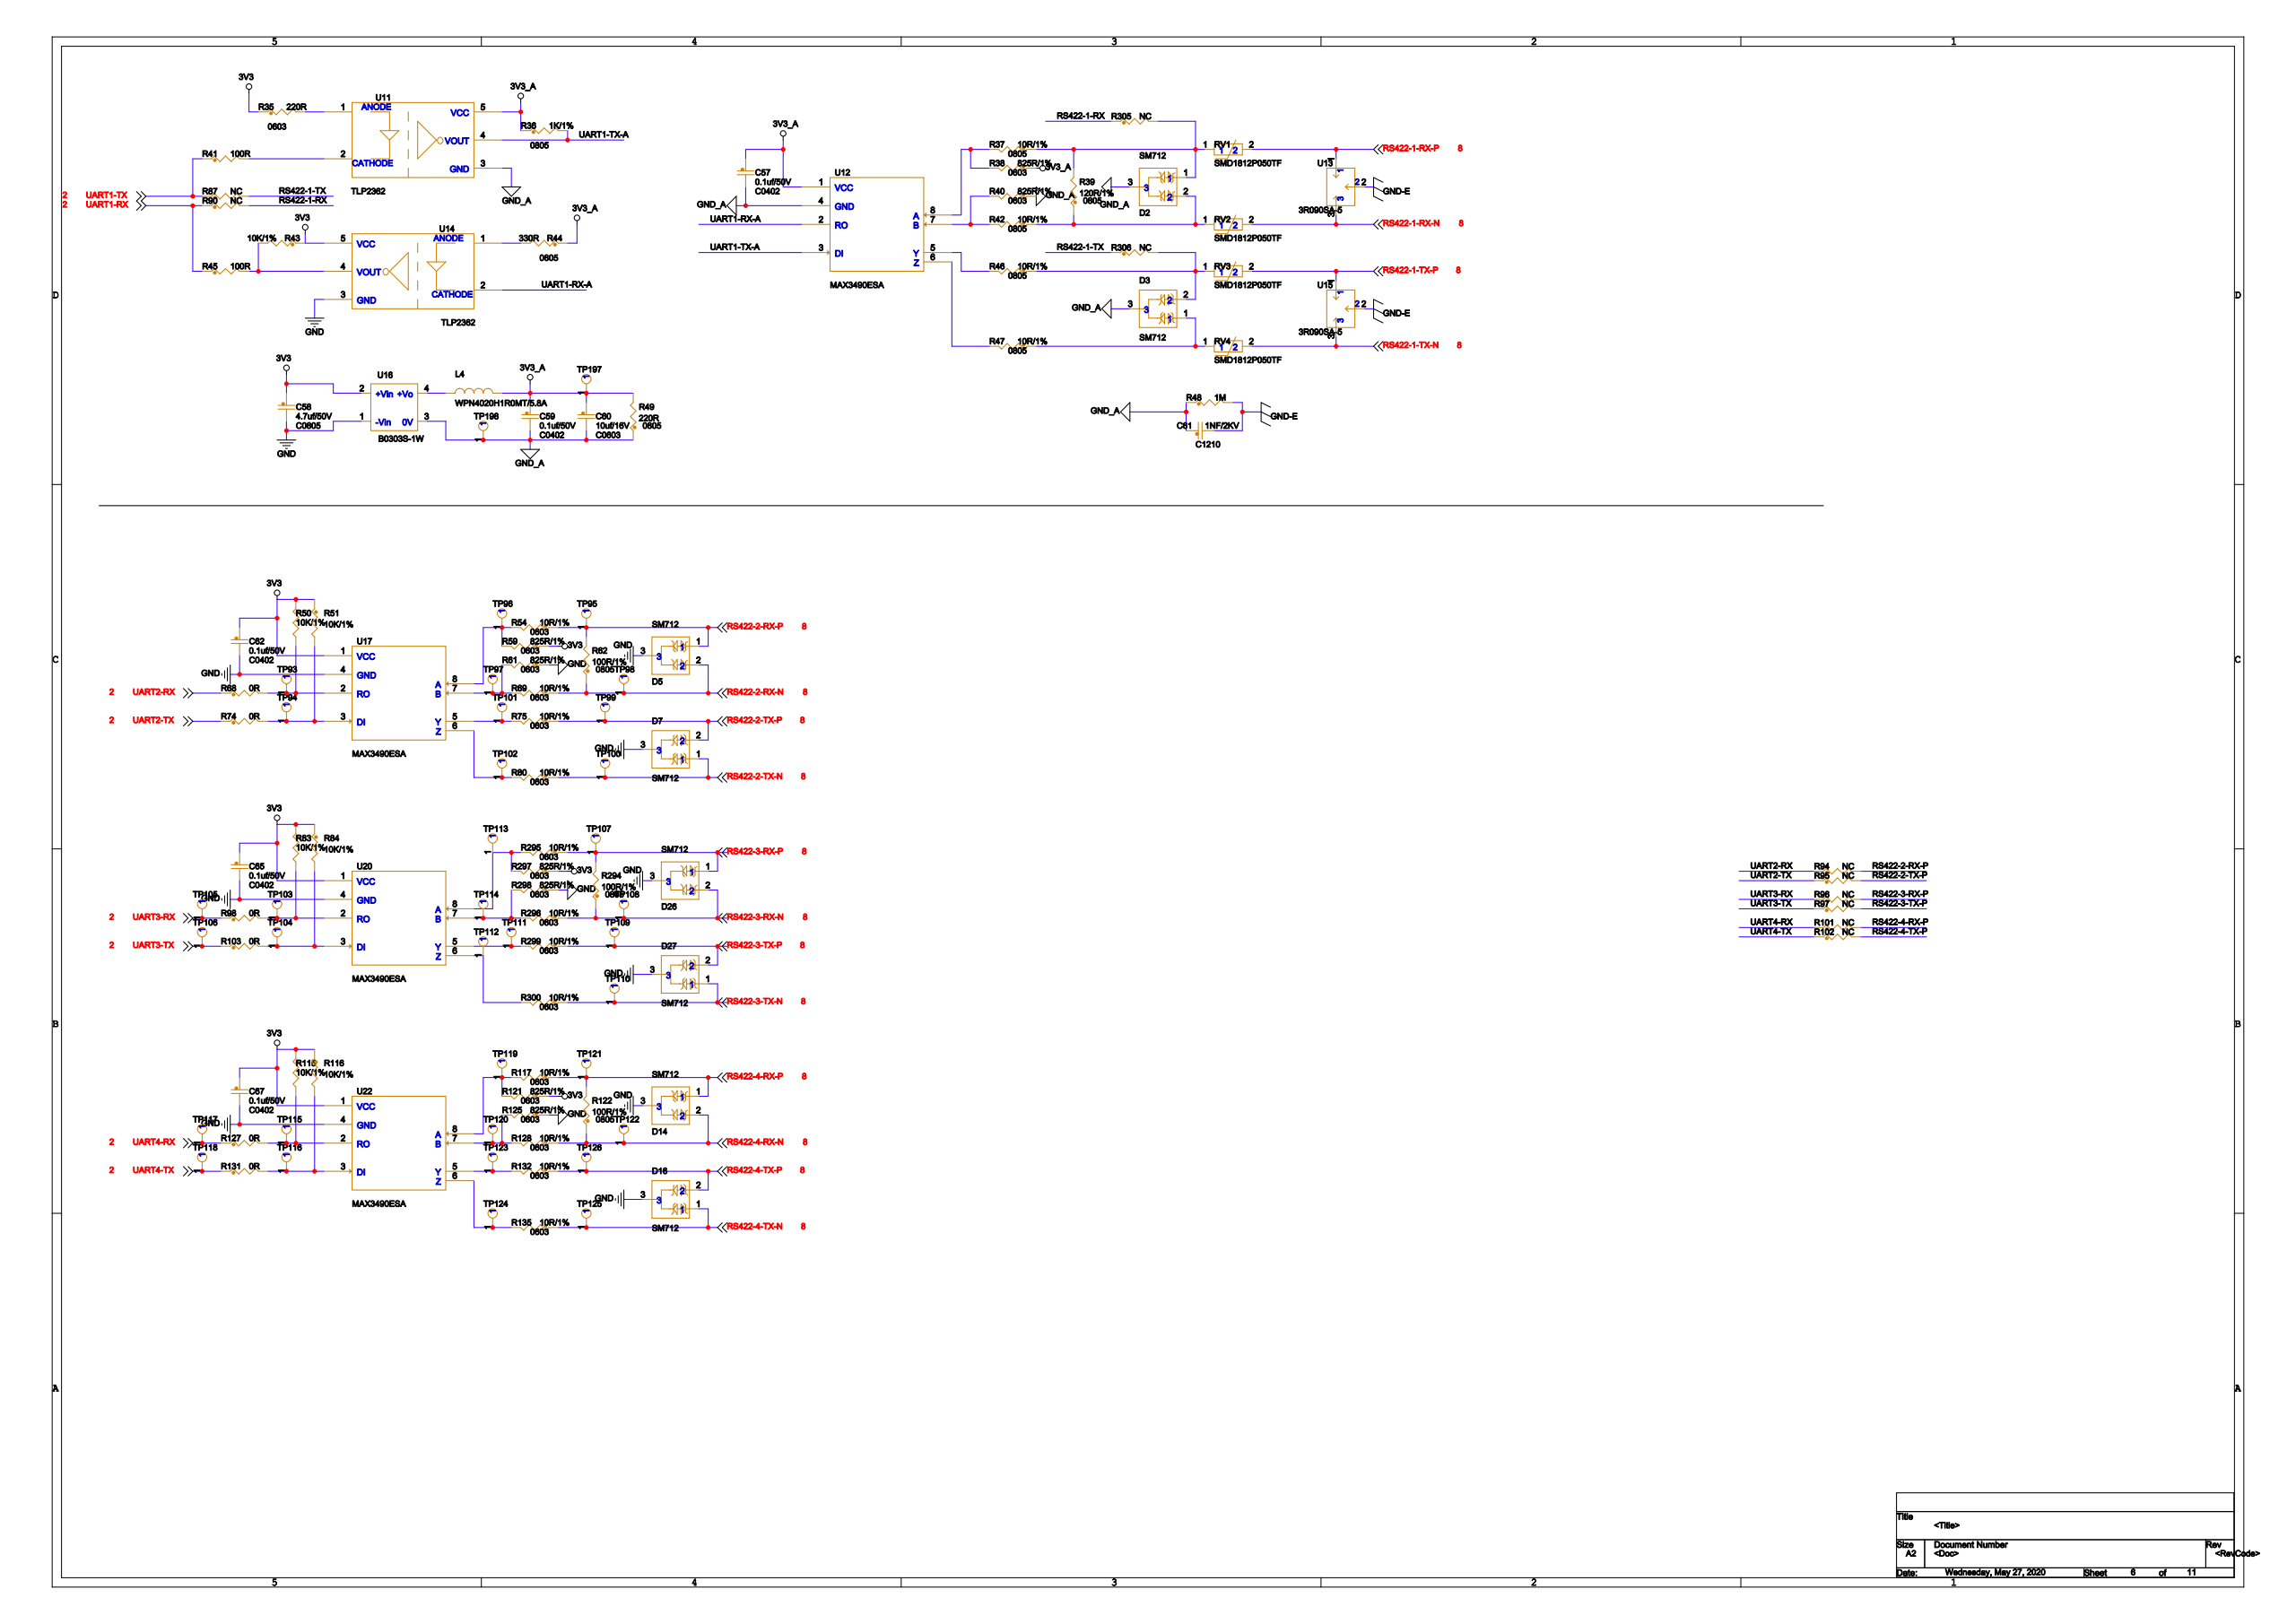Circuit board | Cadence Allegro | 521 parts | 239 nets | one sheet of the schematic
Parts on this sheet (reference | value | footprint):
C57 | 0.1uf/50V | C0402
C58 | 4.7uf/50V | C0805
C59 | 0.1uf/50V | C0402
C60 | 10uf/16V | C0603
C61 | 1NF/2KV | C1210
C62 | 0.1uf/50V | C0402
C65 | 0.1uf/50V | C0402
C67 | 0.1uf/50V | C0402
D2 | SM712 | SOT23
D3 | SM712 | SOT23
D5 | SM712 | SOT23
D7 | SM712 | SOT23
D14 | SM712 | SOT23
D16 | SM712 | SOT23
D26 | SM712 | SOT23
D27 | SM712 | SOT23
L4 | WPN4020H1R0MT/5.8A | SM_IND_4
R35 | 220R | 0603
R36 | 1K/1% | 0805
R37 | 10R/1% | 0805
R38 | 825R/1% | 0603
R39 | 120R/1% | 0805
R40 | 825R/1% | 0603
R41 | 100R | 0603
R42 | 10R/1% | 0805
R43 | 10K/1% | 0402
R44 | 330R | 0805
R45 | 100R | 0603
R46 | 10R/1% | 0805
R47 | 10R/1% | 0805
R48 | 1M | 1206
R49 | 220R | 0805
R50 | 10K/1% | 0402
R51 | 10K/1% | 0402
R54 | 10R/1% | 0603
R59 | 825R/1% | 0603
R61 | 825R/1% | 0603
R62 | 100R/1% | 0805
R68 | 0R | 0603
R69 | 10R/1% | 0603
R74 | 0R | 0603
R75 | 10R/1% | 0603
R80 | 10R/1% | 0603
R83 | 10K/1% | 0402
R84 | 10K/1% | 0402
R87 | NC | 0603
R90 | NC | 0603
R94 | NC | 0603
R95 | NC | 0603
R96 | NC | 0603
R97 | NC | 0603
R98 | 0R | 0603
R101 | NC | 0603
R102 | NC | 0603
R103 | 0R | 0603
R115 | 10K/1% | 0402
R116 | 10K/1% | 0402
R117 | 10R/1% | 0603
R121 | 825R/1% | 0603
R122 | 100R/1% | 0805
R125 | 825R/1% | 0603
R127 | 0R | 0603
R128 | 10R/1% | 0603
R131 | 0R | 0603
R132 | 10R/1% | 0603
R135 | 10R/1% | 0603
R294 | 100R/1% | 0805
R295 | 10R/1% | 0603
R296 | 10R/1% | 0603
R297 | 825R/1% | 0603
R298 | 825R/1% | 0603
R299 | 10R/1% | 0603
R300 | 10R/1% | 0603
R305 | NC | 0603
R306 | NC | 0603
RV1 | SMD1812P050TF | 1812_2
RV2 | SMD1812P050TF | 1812_2
RV3 | SMD1812P050TF | 1812_2
RV4 | SMD1812P050TF | 1812_2
TP93 | TESTPOINT | TESTPOINT-33MIL
TP94 | TESTPOINT | TESTPOINT-33MIL
TP95 | TESTPOINT | TESTPOINT-33MIL
TP96 | TESTPOINT | TESTPOINT-33MIL
TP97 | TESTPOINT | TESTPOINT-33MIL
TP98 | TESTPOINT | TESTPOINT-33MIL
TP99 | TESTPOINT | TESTPOINT-33MIL
TP100 | TESTPOINT | TESTPOINT-33MIL
TP101 | TESTPOINT | TESTPOINT-33MIL
TP102 | TESTPOINT | TESTPOINT-33MIL
TP103 | TESTPOINT | TESTPOINT-33MIL
TP104 | TESTPOINT | TESTPOINT-33MIL
TP105 | TESTPOINT | TESTPOINT-33MIL
TP106 | TESTPOINT | TESTPOINT-33MIL
TP107 | TESTPOINT | TESTPOINT-33MIL
TP108 | TESTPOINT | TESTPOINT-33MIL
TP109 | TESTPOINT | TESTPOINT-33MIL
TP110 | TESTPOINT | TESTPOINT-33MIL
TP111 | TESTPOINT | TESTPOINT-33MIL
TP112 | TESTPOINT | TESTPOINT-33MIL
TP113 | TESTPOINT | TESTPOINT-33MIL
TP114 | TESTPOINT | TESTPOINT-33MIL
TP115 | TESTPOINT | TESTPOINT-33MIL
TP116 | TESTPOINT | TESTPOINT-33MIL
TP117 | TESTPOINT | TESTPOINT-33MIL
TP118 | TESTPOINT | TESTPOINT-33MIL
TP119 | TESTPOINT | TESTPOINT-33MIL
TP120 | TESTPOINT | TESTPOINT-33MIL
TP121 | TESTPOINT | TESTPOINT-33MIL
TP122 | TESTPOINT | TESTPOINT-33MIL
TP123 | TESTPOINT | TESTPOINT-33MIL
TP124 | TESTPOINT | TESTPOINT-33MIL
TP125 | TESTPOINT | TESTPOINT-33MIL
TP126 | TESTPOINT | TESTPOINT-33MIL
TP197 | TESTPOINT | TESTPOINT-33MIL
TP198 | TESTPOINT | TESTPOINT-33MIL
U11 | TLP2362 | TLP2362
U12 | MAX3490ESA | SOP8
U13 | 3R090SA-5 | 3R090SA-5
U14 | TLP2362 | TLP2362
U15 | 3R090SA-5 | 3R090SA-5
U16 | B0303S-1W | B0303S
U17 | MAX3490ESA | SOP8
U20 | MAX3490ESA | SOP8
U22 | MAX3490ESA | SOP8
Nets of these parts (net: part-pin ...):
GND: C58-2 C62-2 C65-2 C67-2 D5-3 D7-3 D14-3 D16-3 D26-3 D27-3 R61-1 R125-1 R298-1 U14-3 U16-1 U17-4 U20-4 U22-4
3V3: C58-1 C62-1 C65-1 C67-1 R35-1 R43-1 R50-1 R51-1 R59-1 R83-1 R84-1 R115-1 R116-1 R121-1 R297-1 U14-5 U16-2 U17-1 U20-1 U22-1
GND-E: C61-2 R48-2 U13-2 U15-2
3V3_A: C57-1 C59-1 C60-1 L4-2 R36-1 R38-1 R44-1 R49-2 TP197-1 U11-5 U12-1
GND_A: C57-2 C59-2 C60-2 C61-1 D2-3 D3-3 R40-1 R48-1 R49-1 TP198-1 U11-3 U12-4 U16-3
RS422-2-TX-N: D7-1 R80-1 TP100-1
N7517990: R75-2 TP101-1 U17-5
N7210093: R80-2 TP102-1 U17-6
N7237292: R83-2 R98-2 TP103-1 U20-2
N7237300: R84-2 R103-2 TP104-1 U20-3
UART3-RX: R96-1 R98-1 TP105-1
UART3-TX: R97-1 R103-1 TP106-1
RS422-3-RX-P: D26-1 R96-2 R294-2 R295-1 TP107-1
RS422-3-RX-N: D26-2 R294-1 R296-1 TP108-1
RS422-3-TX-P: D27-2 R97-2 R299-1 TP109-1
RS422-3-TX-N: D27-1 R300-1 TP110-1
N7800107: R299-2 TP111-1 U20-5
N7799845: R300-2 TP112-1 U20-6
N7237352: R295-2 R297-2 TP113-1 U20-8
N7800141: R296-2 R298-2 TP114-1 U20-7
N7238174: R115-2 R127-2 TP115-1 U22-2
N7238182: R116-2 R131-2 TP116-1 U22-3
UART4-RX: R101-1 R127-1 TP117-1
UART4-TX: R102-1 R131-1 TP118-1
N7520428: R117-2 R121-2 TP119-1 U22-8
N7520728: R125-2 R128-2 TP120-1 U22-7
RS422-4-RX-P: D14-1 R101-2 R117-1 R122-2 TP121-1
RS422-4-RX-N: D14-2 R122-1 R128-1 TP122-1
N7520694: R132-2 TP123-1 U22-5
N7520432: R135-2 TP124-1 U22-6
RS422-4-TX-N: D16-1 R135-1 TP125-1
RS422-4-TX-P: D16-2 R102-2 R132-1 TP126-1
N7211826: R50-2 R68-2 TP93-1 U17-2
N7212000: R51-2 R74-2 TP94-1 U17-3
RS422-2-RX-P: D5-1 R54-1 R62-2 R94-2 TP95-1
N7209761: R54-2 R59-2 TP96-1 U17-8
N7209765: R61-2 R69-2 TP97-1 U17-7
RS422-2-RX-N: D5-2 R62-1 R69-1 TP98-1
RS422-2-TX-P: D7-2 R75-1 R95-2 TP99-1
N7205072: R35-2 U11-1
UART1-TX: R41-1 R87-1
N7205076: R41-2 U11-2
UART1-RX: R45-1 R90-1
N7205694: R43-2 R45-2 U14-4
UART1-TX-A: R36-2 U11-4 U12-3
N7201437: R37-2 R38-2 U12-8
N7201439: R40-2 R42-2 U12-7
RS422-1-RX-P: RV1-2 U13-1
RS422-1-RX-N: RV2-2 U13-3
RS422-1-TX-P: RV3-2 U15-1
RS422-1-TX-N: RV4-2 U15-3
N7205756: R44-2 U14-1
UART1-RX-A: U12-2 U14-2
N7512808: D2-1 R37-1 R39-2 R305-2 RV1-1
N7512812: D2-2 R39-1 R42-1 RV2-1
N7512998: D3-1 R47-1 RV4-1
N7513078: D3-2 R46-1 R306-2 RV3-1
N7208740: L4-1 U16-4
N7202907: R46-2 U12-5
N7202920: R47-2 U12-6
RS422-1-RX: R90-2 R305-1
RS422-1-TX: R87-2 R306-1
UART2-RX: R68-1 R94-1
UART2-TX: R74-1 R95-1